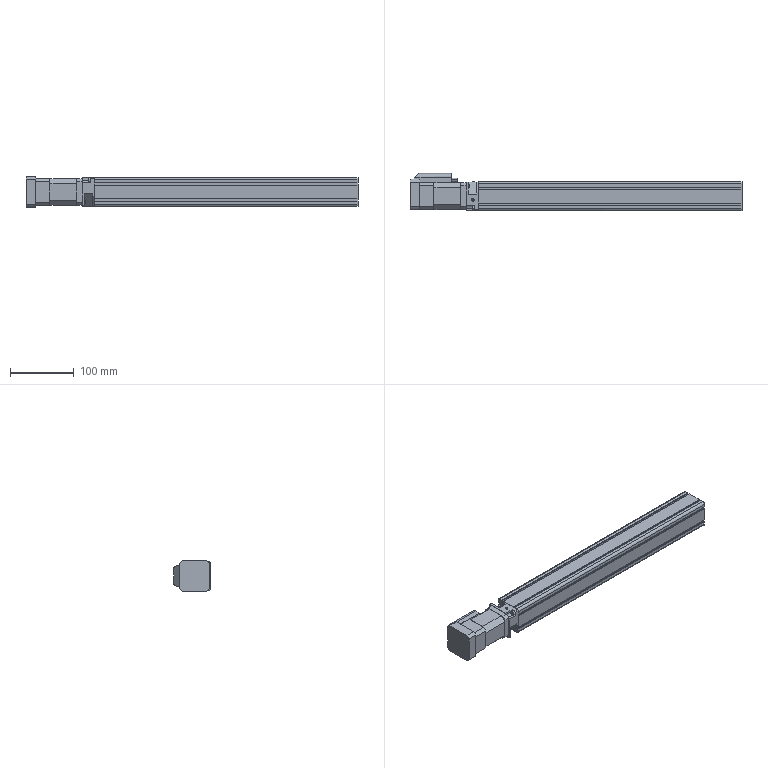Part | STEP file | Guide wheel mechanism revised.sldasm-Part-468 | 1 solid | 269 faces | box 520.5 x 58 x 48 mm | volume 861583 mm3 | plane 193 | cylinder 40 | cone 36 | commonest cylinder face diameters 3.242 x14 7 x8 5.5 x4 6 x4 57.9 x4 8 x2